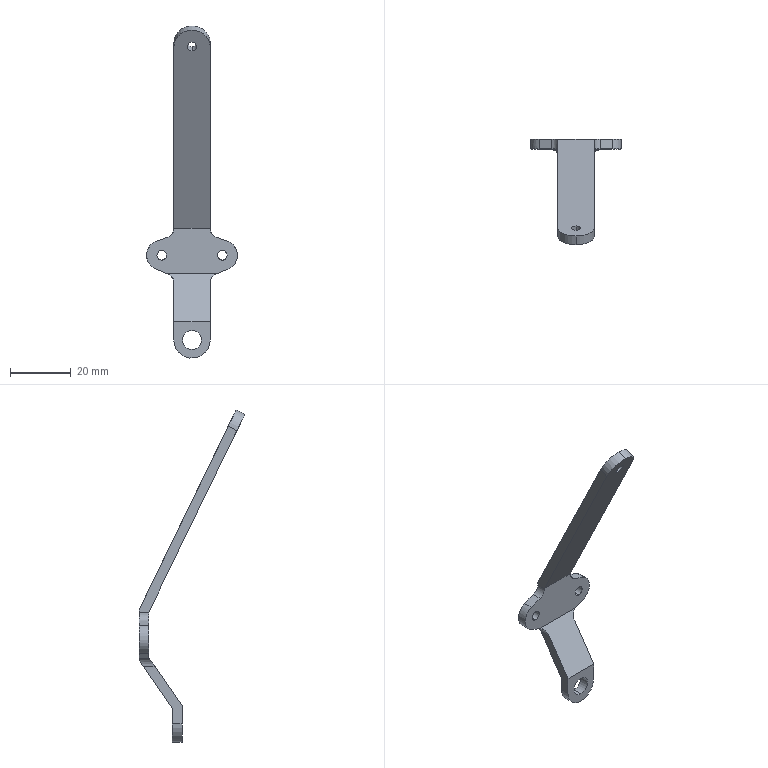Part | SolidWorks | features BaseBody 1 | 1 solid | 33 faces | box 30 x 34.955 x 109.796 mm | volume 4900 mm3 | cylinder 17 | plane 16 | commonest cylinder face diameters 3.2 x6 6 x4 12 x3 6.261 x2 10 x2
STEP:
#1=CARTESIAN_POINT('',(0.,-11.,-24.87));
#2=VERTEX_POINT('',#1);
#3=CARTESIAN_POINT('',(0.,-11.,-31.13));
#4=VERTEX_POINT('',#3);
#5=CARTESIAN_POINT('',(0.,-11.,-28.));
#6=DIRECTION('',(0.,-1.,0.));
#7=DIRECTION('',(0.,0.,1.));
#8=AXIS2_PLACEMENT_3D('',#5,#6,#7);
#9=CIRCLE('',#8,3.13);
#10=EDGE_CURVE('',#2,#4,#9,.T.);
#11=ORIENTED_EDGE('',*,*,#10,.T.);
#12=CARTESIAN_POINT('',(0.,-7.8,-31.13));
#13=VERTEX_POINT('',#12);
#14=CARTESIAN_POINT('',(0.,-11.,-31.13));
#15=DIRECTION('',(0.,1.,0.));
#16=VECTOR('',#15,1000.);
#17=LINE('',#14,#16);
#18=EDGE_CURVE('',#4,#13,#17,.T.);
#19=ORIENTED_EDGE('',*,*,#18,.T.);
#20=CARTESIAN_POINT('',(0.,-7.8,-24.87));
#21=VERTEX_POINT('',#20);
#22=CARTESIAN_POINT('',(0.,-7.8,-28.));
#23=DIRECTION('',(0.,1.,0.));
#24=DIRECTION('',(0.,0.,1.));
#25=AXIS2_PLACEMENT_3D('',#22,#23,#24);
#26=CIRCLE('',#25,3.13);
#27=EDGE_CURVE('',#13,#21,#26,.T.);
#28=ORIENTED_EDGE('',*,*,#27,.T.);
#29=CARTESIAN_POINT('',(0.,-11.,-24.87));
#30=DIRECTION('',(0.,1.,0.));
#31=VECTOR('',#30,1000.);
#32=LINE('',#29,#31);
#33=EDGE_CURVE('',#2,#21,#32,.T.);
#34=ORIENTED_EDGE('',*,*,#33,.F.);
#35=EDGE_LOOP('',(#11,#19,#28,#34));
#36=FACE_OUTER_BOUND('',#35,.T.);
#37=CARTESIAN_POINT('',(0.,-11.,-28.));
#38=DIRECTION('',(0.,1.,0.));
#39=DIRECTION('',(0.,0.,1.));
#40=AXIS2_PLACEMENT_3D('',#37,#38,#39);
#41=CYLINDRICAL_SURFACE('',#40,3.13);
#42=ADVANCED_FACE('',(#36),#41,.F.);
#43=CARTESIAN_POINT('',(-10.,0.,1.6));
#44=VERTEX_POINT('',#43);
#45=CARTESIAN_POINT('',(-10.,0.,-1.6));
#46=VERTEX_POINT('',#45);
#47=CARTESIAN_POINT('',(-10.,0.,1.6));
#48=CARTESIAN_POINT('',(-13.2,0.,1.6));
#49=CARTESIAN_POINT('',(-13.2,0.,-1.6));
#50=CARTESIAN_POINT('',(-10.,0.,-1.6));
#51=(BOUNDED_CURVE()B_SPLINE_CURVE(3,(#47,#48,#49,#50),.UNSPECIFIED.,.F.,.F.)B_SPLINE_CURVE_WITH_KNOTS((4,4),(0.,3.142),.UNSPECIFIED.)CURVE()GEOMETRIC_REPRESENTATION_ITEM()RATIONAL_B_SPLINE_CURVE((1.,0.3333,0.3333,1.))REPRESENTATION_ITEM(''));
#52=EDGE_CURVE('',#44,#46,#51,.T.);
#53=ORIENTED_EDGE('',*,*,#52,.T.);
#54=CARTESIAN_POINT('',(-10.,3.193,-1.596));
#55=VERTEX_POINT('',#54);
#56=CARTESIAN_POINT('',(-10.,-0.01916,-1.6));
#57=DIRECTION('',(0.,1.,0.001373));
#58=VECTOR('',#57,1000.);
#59=LINE('',#56,#58);
#60=EDGE_CURVE('',#46,#55,#59,.T.);
#61=ORIENTED_EDGE('',*,*,#60,.T.);
#62=CARTESIAN_POINT('',(-10.,3.188,1.604));
#63=VERTEX_POINT('',#62);
#64=CARTESIAN_POINT('',(-10.,3.19,0.004381));
#65=DIRECTION('',(0.,1.,0.001373));
#66=DIRECTION('',(0.,-0.001373,1.));
#67=AXIS2_PLACEMENT_3D('',#64,#65,#66);
#68=CIRCLE('',#67,1.6);
#69=EDGE_CURVE('',#55,#63,#68,.T.);
#70=ORIENTED_EDGE('',*,*,#69,.T.);
#71=CARTESIAN_POINT('',(-10.,-0.02355,1.6));
#72=DIRECTION('',(0.,1.,0.001373));
#73=VECTOR('',#72,1000.);
#74=LINE('',#71,#73);
#75=EDGE_CURVE('',#44,#63,#74,.T.);
#76=ORIENTED_EDGE('',*,*,#75,.F.);
#77=EDGE_LOOP('',(#53,#61,#70,#76));
#78=FACE_OUTER_BOUND('',#77,.T.);
#79=CARTESIAN_POINT('',(-10.,-0.02135,-0.00002932));
#80=DIRECTION('',(0.,1.,0.001373));
#81=DIRECTION('',(0.,-0.001373,1.));
#82=AXIS2_PLACEMENT_3D('',#79,#80,#81);
#83=CYLINDRICAL_SURFACE('',#82,1.6);
#84=ADVANCED_FACE('',(#78),#83,.F.);
#85=CARTESIAN_POINT('',(10.,0.,1.6));
#86=VERTEX_POINT('',#85);
#87=CARTESIAN_POINT('',(10.,0.,-1.6));
#88=VERTEX_POINT('',#87);
#89=CARTESIAN_POINT('',(10.,0.,1.6));
#90=CARTESIAN_POINT('',(6.8,0.,1.6));
#91=CARTESIAN_POINT('',(6.8,0.,-1.6));
#92=CARTESIAN_POINT('',(10.,0.,-1.6));
#93=(BOUNDED_CURVE()B_SPLINE_CURVE(3,(#89,#90,#91,#92),.UNSPECIFIED.,.F.,.F.)B_SPLINE_CURVE_WITH_KNOTS((4,4),(0.,3.142),.UNSPECIFIED.)CURVE()GEOMETRIC_REPRESENTATION_ITEM()RATIONAL_B_SPLINE_CURVE((1.,0.3333,0.3333,1.))REPRESENTATION_ITEM(''));
#94=EDGE_CURVE('',#86,#88,#93,.T.);
#95=ORIENTED_EDGE('',*,*,#94,.T.);
#96=CARTESIAN_POINT('',(10.,3.193,-1.596));
#97=VERTEX_POINT('',#96);
#98=CARTESIAN_POINT('',(10.,-0.01916,-1.6));
#99=DIRECTION('',(0.,1.,0.001373));
#100=VECTOR('',#99,1000.);
#101=LINE('',#98,#100);
#102=EDGE_CURVE('',#88,#97,#101,.T.);
#103=ORIENTED_EDGE('',*,*,#102,.T.);
#104=CARTESIAN_POINT('',(10.,3.188,1.604));
#105=VERTEX_POINT('',#104);
#106=CARTESIAN_POINT('',(10.,3.19,0.004381));
#107=DIRECTION('',(0.,1.,0.001373));
#108=DIRECTION('',(0.,-0.001373,1.));
#109=AXIS2_PLACEMENT_3D('',#106,#107,#108);
#110=CIRCLE('',#109,1.6);
#111=EDGE_CURVE('',#97,#105,#110,.T.);
#112=ORIENTED_EDGE('',*,*,#111,.T.);
#113=CARTESIAN_POINT('',(10.,-0.02355,1.6));
#114=DIRECTION('',(0.,1.,0.001373));
#115=VECTOR('',#114,1000.);
#116=LINE('',#113,#115);
#117=EDGE_CURVE('',#86,#105,#116,.T.);
#118=ORIENTED_EDGE('',*,*,#117,.F.);
#119=EDGE_LOOP('',(#95,#103,#112,#118));
#120=FACE_OUTER_BOUND('',#119,.T.);
#121=CARTESIAN_POINT('',(10.,-0.02135,-0.00002932));
#122=DIRECTION('',(0.,1.,0.001373));
#123=DIRECTION('',(0.,-0.001373,1.));
#124=AXIS2_PLACEMENT_3D('',#121,#122,#123);
#125=CYLINDRICAL_SURFACE('',#124,1.6);
#126=ADVANCED_FACE('',(#120),#125,.F.);
#127=CARTESIAN_POINT('',(0.,-29.834,70.44));
#128=VERTEX_POINT('',#127);
#129=CARTESIAN_POINT('',(0.,-28.436,67.561));
#130=VERTEX_POINT('',#129);
#131=CARTESIAN_POINT('',(0.,-29.135,69.001));
#132=DIRECTION('',(0.,-0.8996,-0.4368));
#133=DIRECTION('',(0.,-0.4368,0.8996));
#134=AXIS2_PLACEMENT_3D('',#131,#132,#133);
#135=CIRCLE('',#134,1.6);
#136=EDGE_CURVE('',#128,#130,#135,.T.);
#137=ORIENTED_EDGE('',*,*,#136,.T.);
#138=CARTESIAN_POINT('',(0.,-25.557,68.959));
#139=VERTEX_POINT('',#138);
#140=CARTESIAN_POINT('',(0.,-28.436,67.561));
#141=DIRECTION('',(0.,0.8996,0.4368));
#142=VECTOR('',#141,1000.);
#143=LINE('',#140,#142);
#144=EDGE_CURVE('',#130,#139,#143,.T.);
#145=ORIENTED_EDGE('',*,*,#144,.T.);
#146=CARTESIAN_POINT('',(0.,-26.955,71.838));
#147=VERTEX_POINT('',#146);
#148=CARTESIAN_POINT('',(0.,-26.256,70.398));
#149=DIRECTION('',(0.,0.8996,0.4368));
#150=DIRECTION('',(0.,-0.4368,0.8996));
#151=AXIS2_PLACEMENT_3D('',#148,#149,#150);
#152=CIRCLE('',#151,1.6);
#153=EDGE_CURVE('',#139,#147,#152,.T.);
#154=ORIENTED_EDGE('',*,*,#153,.T.);
#155=CARTESIAN_POINT('',(0.,-29.834,70.44));
#156=DIRECTION('',(0.,0.8996,0.4368));
#157=VECTOR('',#156,1000.);
#158=LINE('',#155,#157);
#159=EDGE_CURVE('',#128,#147,#158,.T.);
#160=ORIENTED_EDGE('',*,*,#159,.F.);
#161=EDGE_LOOP('',(#137,#145,#154,#160));
#162=FACE_OUTER_BOUND('',#161,.T.);
#163=CARTESIAN_POINT('',(0.,-29.135,69.001));
#164=DIRECTION('',(0.,0.8996,0.4368));
#165=DIRECTION('',(0.,-0.4368,0.8996));
#166=AXIS2_PLACEMENT_3D('',#163,#164,#165);
#167=CYLINDRICAL_SURFACE('',#166,1.6);
#168=ADVANCED_FACE('',(#162),#167,.F.);
#169=CARTESIAN_POINT('',(-6.,-29.135,69.001));
#170=VERTEX_POINT('',#169);
#171=CARTESIAN_POINT('',(0.,-31.755,74.398));
#172=VERTEX_POINT('',#171);
#173=CARTESIAN_POINT('',(0.,-29.135,69.001));
#174=DIRECTION('',(0.,0.8996,0.4368));
#175=DIRECTION('',(0.,-0.4368,0.8996));
#176=AXIS2_PLACEMENT_3D('',#173,#174,#175);
#177=CIRCLE('',#176,6.);
#178=EDGE_CURVE('',#170,#172,#177,.T.);
#179=ORIENTED_EDGE('',*,*,#178,.T.);
#180=CARTESIAN_POINT('',(0.,-28.877,75.796));
#181=VERTEX_POINT('',#180);
#182=CARTESIAN_POINT('',(0.,-31.755,74.398));
#183=DIRECTION('',(0.,0.8996,0.4368));
#184=VECTOR('',#183,1000.);
#185=LINE('',#182,#184);
#186=EDGE_CURVE('',#172,#181,#185,.T.);
#187=ORIENTED_EDGE('',*,*,#186,.T.);
#188=CARTESIAN_POINT('',(-6.,-26.256,70.398));
#189=VERTEX_POINT('',#188);
#190=CARTESIAN_POINT('',(0.,-26.256,70.398));
#191=DIRECTION('',(0.,-0.8996,-0.4368));
#192=DIRECTION('',(0.,-0.4368,0.8996));
#193=AXIS2_PLACEMENT_3D('',#190,#191,#192);
#194=CIRCLE('',#193,6.);
#195=EDGE_CURVE('',#181,#189,#194,.T.);
#196=ORIENTED_EDGE('',*,*,#195,.T.);
#197=CARTESIAN_POINT('',(-6.,-29.135,69.001));
#198=DIRECTION('',(0.,0.8996,0.4368));
#199=VECTOR('',#198,1000.);
#200=LINE('',#197,#199);
#201=EDGE_CURVE('',#170,#189,#200,.T.);
#202=ORIENTED_EDGE('',*,*,#201,.F.);
#203=EDGE_LOOP('',(#179,#187,#196,#202));
#204=FACE_OUTER_BOUND('',#203,.T.);
#205=CARTESIAN_POINT('',(0.,-29.135,69.001));
#206=DIRECTION('',(0.,0.8996,0.4368));
#207=DIRECTION('',(0.,-0.4368,0.8996));
#208=AXIS2_PLACEMENT_3D('',#205,#206,#207);
#209=CYLINDRICAL_SURFACE('',#208,6.);
#210=ADVANCED_FACE('',(#204),#209,.T.);
#211=ORIENTED_EDGE('',*,*,#18,.F.);
#212=CARTESIAN_POINT('',(0.,-11.,-28.));
#213=DIRECTION('',(0.,-1.,0.));
#214=DIRECTION('',(0.,0.,1.));
#215=AXIS2_PLACEMENT_3D('',#212,#213,#214);
#216=CIRCLE('',#215,3.13);
#217=EDGE_CURVE('',#4,#2,#216,.T.);
#218=ORIENTED_EDGE('',*,*,#217,.T.);
#219=ORIENTED_EDGE('',*,*,#33,.T.);
#220=CARTESIAN_POINT('',(0.,-7.8,-28.));
#221=DIRECTION('',(0.,1.,0.));
#222=DIRECTION('',(0.,0.,1.));
#223=AXIS2_PLACEMENT_3D('',#220,#221,#222);
#224=CIRCLE('',#223,3.13);
#225=EDGE_CURVE('',#21,#13,#224,.T.);
#226=ORIENTED_EDGE('',*,*,#225,.T.);
#227=EDGE_LOOP('',(#211,#218,#219,#226));
#228=FACE_OUTER_BOUND('',#227,.T.);
#229=CARTESIAN_POINT('',(0.,-11.,-28.));
#230=DIRECTION('',(0.,1.,0.));
#231=DIRECTION('',(0.,0.,1.));
#232=AXIS2_PLACEMENT_3D('',#229,#230,#231);
#233=CYLINDRICAL_SURFACE('',#232,3.13);
#234=ADVANCED_FACE('',(#228),#233,.F.);
#235=ORIENTED_EDGE('',*,*,#225,.F.);
#236=ORIENTED_EDGE('',*,*,#27,.F.);
#237=EDGE_LOOP('',(#235,#236));
#238=FACE_BOUND('',#237,.T.);
#239=CARTESIAN_POINT('',(-6.,-7.8,-22.994));
#240=VERTEX_POINT('',#239);
#241=CARTESIAN_POINT('',(-6.,-7.8,-28.));
#242=VERTEX_POINT('',#241);
#243=CARTESIAN_POINT('',(-6.,-7.8,-28.53));
#244=DIRECTION('',(0.,0.,-1.));
#245=VECTOR('',#244,1000.);
#246=LINE('',#243,#245);
#247=EDGE_CURVE('',#240,#242,#246,.T.);
#248=ORIENTED_EDGE('',*,*,#247,.F.);
#249=CARTESIAN_POINT('',(6.,-7.8,-22.994));
#250=VERTEX_POINT('',#249);
#251=CARTESIAN_POINT('',(0.,-7.8,-22.994));
#252=DIRECTION('',(-1.,0.,0.));
#253=VECTOR('',#252,1000.);
#254=LINE('',#251,#253);
#255=EDGE_CURVE('',#250,#240,#254,.T.);
#256=ORIENTED_EDGE('',*,*,#255,.F.);
#257=CARTESIAN_POINT('',(6.,-7.8,-28.));
#258=VERTEX_POINT('',#257);
#259=CARTESIAN_POINT('',(6.,-7.8,-28.53));
#260=DIRECTION('',(0.,0.,1.));
#261=VECTOR('',#260,1000.);
#262=LINE('',#259,#261);
#263=EDGE_CURVE('',#258,#250,#262,.T.);
#264=ORIENTED_EDGE('',*,*,#263,.F.);
#265=CARTESIAN_POINT('',(0.,-7.8,-28.));
#266=DIRECTION('',(0.,-1.,0.));
#267=DIRECTION('',(0.,0.,1.));
#268=AXIS2_PLACEMENT_3D('',#265,#266,#267);
#269=CIRCLE('',#268,6.);
#270=EDGE_CURVE('',#242,#258,#269,.T.);
#271=ORIENTED_EDGE('',*,*,#270,.F.);
#272=EDGE_LOOP('',(#248,#256,#264,#271));
#273=FACE_OUTER_BOUND('',#272,.T.);
#274=CARTESIAN_POINT('',(-6.,-7.8,-22.994));
#275=DIRECTION('',(0.,-1.,0.));
#276=DIRECTION('',(0.,0.,-1.));
#277=AXIS2_PLACEMENT_3D('',#274,#275,#276);
#278=PLANE('',#277);
#279=ADVANCED_FACE('',(#238,#273),#278,.F.);
#280=ORIENTED_EDGE('',*,*,#10,.F.);
#281=ORIENTED_EDGE('',*,*,#217,.F.);
#282=EDGE_LOOP('',(#280,#281));
#283=FACE_BOUND('',#282,.T.);
#284=CARTESIAN_POINT('',(6.,-11.,-28.));
#285=VERTEX_POINT('',#284);
#286=CARTESIAN_POINT('',(-6.,-11.,-28.));
#287=VERTEX_POINT('',#286);
#288=CARTESIAN_POINT('',(0.,-11.,-28.));
#289=DIRECTION('',(0.,1.,0.));
#290=DIRECTION('',(0.,0.,1.));
#291=AXIS2_PLACEMENT_3D('',#288,#289,#290);
#292=CIRCLE('',#291,6.);
#293=EDGE_CURVE('',#285,#287,#292,.T.);
#294=ORIENTED_EDGE('',*,*,#293,.F.);
#295=CARTESIAN_POINT('',(6.,-11.,-22.));
#296=VERTEX_POINT('',#295);
#297=CARTESIAN_POINT('',(6.,-11.,-28.036));
#298=DIRECTION('',(0.,0.,-1.));
#299=VECTOR('',#298,1000.);
#300=LINE('',#297,#299);
#301=EDGE_CURVE('',#296,#285,#300,.T.);
#302=ORIENTED_EDGE('',*,*,#301,.F.);
#303=CARTESIAN_POINT('',(-6.,-11.,-22.));
#304=VERTEX_POINT('',#303);
#305=CARTESIAN_POINT('',(0.,-11.,-22.));
#306=DIRECTION('',(1.,0.,0.));
#307=VECTOR('',#306,1000.);
#308=LINE('',#305,#307);
#309=EDGE_CURVE('',#304,#296,#308,.T.);
#310=ORIENTED_EDGE('',*,*,#309,.F.);
#311=CARTESIAN_POINT('',(-6.,-11.,-28.036));
#312=DIRECTION('',(0.,0.,1.));
#313=VECTOR('',#312,1000.);
#314=LINE('',#311,#313);
#315=EDGE_CURVE('',#287,#304,#314,.T.);
#316=ORIENTED_EDGE('',*,*,#315,.F.);
#317=EDGE_LOOP('',(#294,#302,#310,#316));
#318=FACE_OUTER_BOUND('',#317,.T.);
#319=CARTESIAN_POINT('',(-6.,-11.,-34.072));
#320=DIRECTION('',(0.,1.,0.));
#321=DIRECTION('',(0.,0.,1.));
#322=AXIS2_PLACEMENT_3D('',#319,#320,#321);
#323=PLANE('',#322);
#324=ADVANCED_FACE('',(#283,#318),#323,.F.);
#325=ORIENTED_EDGE('',*,*,#270,.T.);
#326=CARTESIAN_POINT('',(6.,-9.4,-28.));
#327=DIRECTION('',(0.,1.,0.));
#328=VECTOR('',#327,1000.);
#329=LINE('',#326,#328);
#330=EDGE_CURVE('',#285,#258,#329,.T.);
#331=ORIENTED_EDGE('',*,*,#330,.F.);
#332=ORIENTED_EDGE('',*,*,#293,.T.);
#333=CARTESIAN_POINT('',(-6.,-9.4,-28.));
#334=DIRECTION('',(0.,-1.,0.));
#335=VECTOR('',#334,1000.);
#336=LINE('',#333,#335);
#337=EDGE_CURVE('',#242,#287,#336,.T.);
#338=ORIENTED_EDGE('',*,*,#337,.F.);
#339=EDGE_LOOP('',(#325,#331,#332,#338));
#340=FACE_OUTER_BOUND('',#339,.T.);
#341=CARTESIAN_POINT('',(0.,-11.,-28.));
#342=DIRECTION('',(0.,1.,0.));
#343=DIRECTION('',(0.,0.,1.));
#344=AXIS2_PLACEMENT_3D('',#341,#342,#343);
#345=CYLINDRICAL_SURFACE('',#344,6.);
#346=ADVANCED_FACE('',(#340),#345,.T.);
#347=CARTESIAN_POINT('',(-6.,1.807,-9.02));
#348=VERTEX_POINT('',#347);
#349=CARTESIAN_POINT('',(-6.,1.807,-9.02));
#350=DIRECTION('',(0.,-0.5665,-0.824));
#351=VECTOR('',#350,1000.);
#352=LINE('',#349,#351);
#353=EDGE_CURVE('',#348,#240,#352,.T.);
#354=ORIENTED_EDGE('',*,*,#353,.T.);
#355=ORIENTED_EDGE('',*,*,#247,.T.);
#356=ORIENTED_EDGE('',*,*,#337,.T.);
#357=ORIENTED_EDGE('',*,*,#315,.T.);
#358=CARTESIAN_POINT('',(-6.,-2.08,-9.025));
#359=VERTEX_POINT('',#358);
#360=CARTESIAN_POINT('',(-6.,-11.,-22.));
#361=DIRECTION('',(0.,0.5665,0.824));
#362=VECTOR('',#361,1000.);
#363=LINE('',#360,#362);
#364=EDGE_CURVE('',#304,#359,#363,.T.);
#365=ORIENTED_EDGE('',*,*,#364,.T.);
#366=CARTESIAN_POINT('',(-6.,-2.08,-9.025));
#367=DIRECTION('',(0.,1.,0.001373));
#368=VECTOR('',#367,1000.);
#369=LINE('',#366,#368);
#370=EDGE_CURVE('',#359,#348,#369,.T.);
#371=ORIENTED_EDGE('',*,*,#370,.T.);
#372=EDGE_LOOP('',(#354,#355,#356,#357,#365,#371));
#373=FACE_OUTER_BOUND('',#372,.T.);
#374=CARTESIAN_POINT('',(-6.,-11.,-28.));
#375=DIRECTION('',(-1.,0.,0.));
#376=DIRECTION('',(0.,0.,1.));
#377=AXIS2_PLACEMENT_3D('',#374,#375,#376);
#378=PLANE('',#377);
#379=ADVANCED_FACE('',(#373),#378,.T.);
#380=CARTESIAN_POINT('',(-6.786,3.2,-6.994));
#381=VERTEX_POINT('',#380);
#382=CARTESIAN_POINT('',(-6.786,3.2,-6.994));
#383=CARTESIAN_POINT('',(-6.274,2.815,-7.554));
#384=CARTESIAN_POINT('',(-6.,2.329,-8.261));
#385=CARTESIAN_POINT('',(-6.,1.807,-9.02));
#386=(BOUNDED_CURVE()B_SPLINE_CURVE(3,(#382,#383,#384,#385),.UNSPECIFIED.,.F.,.F.)B_SPLINE_CURVE_WITH_KNOTS((4,4),(0.8303,1.571),.UNSPECIFIED.)CURVE()GEOMETRIC_REPRESENTATION_ITEM()RATIONAL_B_SPLINE_CURVE((1.,0.9548,0.9548,1.))REPRESENTATION_ITEM(''));
#387=EDGE_CURVE('',#381,#348,#386,.T.);
#388=ORIENTED_EDGE('',*,*,#387,.F.);
#389=CARTESIAN_POINT('',(6.786,3.2,-6.994));
#390=VERTEX_POINT('',#389);
#391=CARTESIAN_POINT('',(0.,3.2,-6.994));
#392=DIRECTION('',(-1.,0.,0.));
#393=VECTOR('',#392,1000.);
#394=LINE('',#391,#393);
#395=EDGE_CURVE('',#390,#381,#394,.T.);
#396=ORIENTED_EDGE('',*,*,#395,.F.);
#397=CARTESIAN_POINT('',(6.,1.807,-9.02));
#398=VERTEX_POINT('',#397);
#399=CARTESIAN_POINT('',(6.,1.807,-9.02));
#400=CARTESIAN_POINT('',(6.,2.329,-8.261));
#401=CARTESIAN_POINT('',(6.274,2.815,-7.554));
#402=CARTESIAN_POINT('',(6.786,3.2,-6.994));
#403=(BOUNDED_CURVE()B_SPLINE_CURVE(3,(#399,#400,#401,#402),.UNSPECIFIED.,.F.,.F.)B_SPLINE_CURVE_WITH_KNOTS((4,4),(4.712,5.453),.UNSPECIFIED.)CURVE()GEOMETRIC_REPRESENTATION_ITEM()RATIONAL_B_SPLINE_CURVE((1.,0.9548,0.9548,1.))REPRESENTATION_ITEM(''));
#404=EDGE_CURVE('',#398,#390,#403,.T.);
#405=ORIENTED_EDGE('',*,*,#404,.F.);
#406=CARTESIAN_POINT('',(6.,-2.3,-14.994));
#407=DIRECTION('',(0.,0.5665,0.824));
#408=VECTOR('',#407,1000.);
#409=LINE('',#406,#408);
#410=EDGE_CURVE('',#250,#398,#409,.T.);
#411=ORIENTED_EDGE('',*,*,#410,.F.);
#412=ORIENTED_EDGE('',*,*,#255,.T.);
#413=ORIENTED_EDGE('',*,*,#353,.F.);
#414=EDGE_LOOP('',(#388,#396,#405,#411,#412,#413));
#415=FACE_OUTER_BOUND('',#414,.T.);
#416=CARTESIAN_POINT('',(-6.867,3.2,-6.994));
#417=DIRECTION('',(0.,-0.824,0.5665));
#418=DIRECTION('',(0.,-0.5665,-0.824));
#419=AXIS2_PLACEMENT_3D('',#416,#417,#418);
#420=PLANE('',#419);
#421=ADVANCED_FACE('',(#415),#420,.F.);
#422=ORIENTED_EDGE('',*,*,#330,.T.);
#423=ORIENTED_EDGE('',*,*,#263,.T.);
#424=ORIENTED_EDGE('',*,*,#410,.T.);
#425=CARTESIAN_POINT('',(6.,-2.08,-9.025));
#426=VERTEX_POINT('',#425);
#427=CARTESIAN_POINT('',(6.,-2.111,-9.025));
#428=DIRECTION('',(0.,1.,0.001373));
#429=VECTOR('',#428,1000.);
#430=LINE('',#427,#429);
#431=EDGE_CURVE('',#426,#398,#430,.T.);
#432=ORIENTED_EDGE('',*,*,#431,.F.);
#433=CARTESIAN_POINT('',(6.,-11.,-22.));
#434=DIRECTION('',(0.,0.5665,0.824));
#435=VECTOR('',#434,1000.);
#436=LINE('',#433,#435);
#437=EDGE_CURVE('',#296,#426,#436,.T.);
#438=ORIENTED_EDGE('',*,*,#437,.F.);
#439=ORIENTED_EDGE('',*,*,#301,.T.);
#440=EDGE_LOOP('',(#422,#423,#424,#432,#438,#439));
#441=FACE_OUTER_BOUND('',#440,.T.);
#442=CARTESIAN_POINT('',(6.,-11.,-28.));
#443=DIRECTION('',(-1.,0.,0.));
#444=DIRECTION('',(0.,0.,1.));
#445=AXIS2_PLACEMENT_3D('',#442,#443,#444);
#446=PLANE('',#445);
#447=ADVANCED_FACE('',(#441),#446,.F.);
#448=ORIENTED_EDGE('',*,*,#309,.T.);
#449=ORIENTED_EDGE('',*,*,#437,.T.);
#450=CARTESIAN_POINT('',(7.882,-0.1639,-6.238));
#451=VERTEX_POINT('',#450);
#452=CARTESIAN_POINT('',(7.882,-0.1639,-6.238));
#453=CARTESIAN_POINT('',(6.708,-0.4882,-6.71));
#454=CARTESIAN_POINT('',(6.,-1.209,-7.759));
#455=CARTESIAN_POINT('',(6.,-2.08,-9.025));
#456=(BOUNDED_CURVE()B_SPLINE_CURVE(3,(#452,#453,#454,#455),.UNSPECIFIED.,.F.,.F.)B_SPLINE_CURVE_WITH_KNOTS((4,4),(0.3818,1.571),.UNSPECIFIED.)CURVE()GEOMETRIC_REPRESENTATION_ITEM()RATIONAL_B_SPLINE_CURVE((1.,0.8856,0.8856,1.))REPRESENTATION_ITEM(''));
#457=EDGE_CURVE('',#451,#426,#456,.T.);
#458=ORIENTED_EDGE('',*,*,#457,.F.);
#459=CARTESIAN_POINT('',(8.476,0.,-6.));
#460=VERTEX_POINT('',#459);
#461=CARTESIAN_POINT('',(7.882,-0.1639,-6.238));
#462=DIRECTION('',(0.8988,0.2483,0.3612));
#463=VECTOR('',#462,1000.);
#464=LINE('',#461,#463);
#465=EDGE_CURVE('',#451,#460,#464,.T.);
#466=ORIENTED_EDGE('',*,*,#465,.T.);
#467=CARTESIAN_POINT('',(-8.476,0.,-6.));
#468=VERTEX_POINT('',#467);
#469=CARTESIAN_POINT('',(0.,0.,-6.));
#470=DIRECTION('',(1.,0.,0.));
#471=VECTOR('',#470,1000.);
#472=LINE('',#469,#471);
#473=EDGE_CURVE('',#468,#460,#472,.T.);
#474=ORIENTED_EDGE('',*,*,#473,.F.);
#475=CARTESIAN_POINT('',(-7.882,-0.1639,-6.238));
#476=VERTEX_POINT('',#475);
#477=CARTESIAN_POINT('',(-7.882,-0.1639,-6.238));
#478=DIRECTION('',(-0.8988,0.2483,0.3612));
#479=VECTOR('',#478,1000.);
#480=LINE('',#477,#479);
#481=EDGE_CURVE('',#476,#468,#480,.T.);
#482=ORIENTED_EDGE('',*,*,#481,.F.);
#483=CARTESIAN_POINT('',(-6.,-2.08,-9.025));
#484=CARTESIAN_POINT('',(-6.,-1.209,-7.759));
#485=CARTESIAN_POINT('',(-6.708,-0.4882,-6.71));
#486=CARTESIAN_POINT('',(-7.882,-0.1639,-6.238));
#487=(BOUNDED_CURVE()B_SPLINE_CURVE(3,(#483,#484,#485,#486),.UNSPECIFIED.,.F.,.F.)B_SPLINE_CURVE_WITH_KNOTS((4,4),(4.712,5.901),.UNSPECIFIED.)CURVE()GEOMETRIC_REPRESENTATION_ITEM()RATIONAL_B_SPLINE_CURVE((1.,0.8856,0.8856,1.))REPRESENTATION_ITEM(''));
#488=EDGE_CURVE('',#359,#476,#487,.T.);
#489=ORIENTED_EDGE('',*,*,#488,.F.);
#490=ORIENTED_EDGE('',*,*,#364,.F.);
#491=EDGE_LOOP('',(#448,#449,#458,#466,#474,#482,#489,#490));
#492=FACE_OUTER_BOUND('',#491,.T.);
#493=CARTESIAN_POINT('',(-8.577,-11.,-22.));
#494=DIRECTION('',(0.,0.824,-0.5665));
#495=DIRECTION('',(0.,0.5665,0.824));
#496=AXIS2_PLACEMENT_3D('',#493,#494,#495);
#497=PLANE('',#496);
#498=ADVANCED_FACE('',(#492),#497,.F.);
#499=CARTESIAN_POINT('',(-7.882,3.199,-6.234));
#500=VERTEX_POINT('',#499);
#501=CARTESIAN_POINT('',(-9.,3.203,-9.018));
#502=DIRECTION('',(0.,1.,0.001373));
#503=DIRECTION('',(0.,-0.001373,1.));
#504=AXIS2_PLACEMENT_3D('',#501,#502,#503);
#505=CIRCLE('',#504,3.);
#506=EDGE_CURVE('',#500,#381,#505,.T.);
#507=ORIENTED_EDGE('',*,*,#506,.T.);
#508=ORIENTED_EDGE('',*,*,#387,.T.);
#509=ORIENTED_EDGE('',*,*,#370,.F.);
#510=ORIENTED_EDGE('',*,*,#488,.T.);
#511=CARTESIAN_POINT('',(-7.882,0.5419,-6.237));
#512=DIRECTION('',(0.,1.,0.001373));
#513=VECTOR('',#512,1000.);
#514=LINE('',#511,#513);
#515=EDGE_CURVE('',#476,#500,#514,.T.);
#516=ORIENTED_EDGE('',*,*,#515,.T.);
#517=EDGE_LOOP('',(#507,#508,#509,#510,#516));
#518=FACE_OUTER_BOUND('',#517,.T.);
#519=CARTESIAN_POINT('',(-9.,-2.111,-9.025));
#520=DIRECTION('',(0.,1.,0.001373));
#521=DIRECTION('',(0.,-0.001373,1.));
#522=AXIS2_PLACEMENT_3D('',#519,#520,#521);
#523=CYLINDRICAL_SURFACE('',#522,3.);
#524=ADVANCED_FACE('',(#518),#523,.F.);
#525=CARTESIAN_POINT('',(-10.,3.19,0.004381));
#526=DIRECTION('',(0.,1.,0.001373));
#527=DIRECTION('',(0.,-0.001373,1.));
#528=AXIS2_PLACEMENT_3D('',#525,#526,#527);
#529=CIRCLE('',#528,1.6);
#530=EDGE_CURVE('',#63,#55,#529,.T.);
#531=ORIENTED_EDGE('',*,*,#530,.F.);
#532=ORIENTED_EDGE('',*,*,#69,.F.);
#533=EDGE_LOOP('',(#531,#532));
#534=FACE_BOUND('',#533,.T.);
#535=CARTESIAN_POINT('',(10.,3.19,0.004381));
#536=DIRECTION('',(0.,1.,0.001373));
#537=DIRECTION('',(0.,-0.001373,1.));
#538=AXIS2_PLACEMENT_3D('',#535,#536,#537);
#539=CIRCLE('',#538,1.6);
#540=EDGE_CURVE('',#105,#97,#539,.T.);
#541=ORIENTED_EDGE('',*,*,#540,.F.);
#542=ORIENTED_EDGE('',*,*,#111,.F.);
#543=EDGE_LOOP('',(#541,#542));
#544=FACE_BOUND('',#543,.T.);
#545=ORIENTED_EDGE('',*,*,#506,.F.);
#546=CARTESIAN_POINT('',(-11.863,3.197,-4.636));
#547=VERTEX_POINT('',#546);
#548=CARTESIAN_POINT('',(-11.863,3.197,-4.636));
#549=DIRECTION('',(0.928,0.0005116,-0.3726));
#550=VECTOR('',#549,1000.);
#551=LINE('',#548,#550);
#552=EDGE_CURVE('',#547,#500,#551,.T.);
#553=ORIENTED_EDGE('',*,*,#552,.F.);
#554=CARTESIAN_POINT('',(-12.184,3.184,4.502));
#555=VERTEX_POINT('',#554);
#556=CARTESIAN_POINT('',(-10.,3.19,0.004381));
#557=DIRECTION('',(0.,-1.,-0.001373));
#558=DIRECTION('',(0.,-0.001373,1.));
#559=AXIS2_PLACEMENT_3D('',#556,#557,#558);
#560=CIRCLE('',#559,5.);
#561=EDGE_CURVE('',#555,#547,#560,.T.);
#562=ORIENTED_EDGE('',*,*,#561,.F.);
#563=CARTESIAN_POINT('',(-8.,3.182,5.981));
#564=VERTEX_POINT('',#563);
#565=CARTESIAN_POINT('',(-8.,3.182,5.981));
#566=DIRECTION('',(-0.9429,0.0004575,-0.3332));
#567=VECTOR('',#566,1000.);
#568=LINE('',#565,#567);
#569=EDGE_CURVE('',#564,#555,#568,.T.);
#570=ORIENTED_EDGE('',*,*,#569,.F.);
#571=CARTESIAN_POINT('',(-6.,3.178,8.809));
#572=VERTEX_POINT('',#571);
#573=CARTESIAN_POINT('',(-9.,3.178,8.809));
#574=DIRECTION('',(0.,1.,0.001373));
#575=DIRECTION('',(0.,-0.001373,1.));
#576=AXIS2_PLACEMENT_3D('',#573,#574,#575);
#577=CIRCLE('',#576,3.);
#578=EDGE_CURVE('',#572,#564,#577,.T.);
#579=ORIENTED_EDGE('',*,*,#578,.F.);
#580=CARTESIAN_POINT('',(-6.,3.177,9.783));
#581=VERTEX_POINT('',#580);
#582=CARTESIAN_POINT('',(-6.,3.177,9.783));
#583=DIRECTION('',(0.,0.001373,-1.));
#584=VECTOR('',#583,1000.);
#585=LINE('',#582,#584);
#586=EDGE_CURVE('',#581,#572,#585,.T.);
#587=ORIENTED_EDGE('',*,*,#586,.F.);
#588=CARTESIAN_POINT('',(6.,3.177,9.783));
#589=VERTEX_POINT('',#588);
#590=CARTESIAN_POINT('',(0.,3.177,9.783));
#591=DIRECTION('',(-1.,0.,0.));
#592=VECTOR('',#591,1000.);
#593=LINE('',#590,#592);
#594=EDGE_CURVE('',#589,#581,#593,.T.);
#595=ORIENTED_EDGE('',*,*,#594,.F.);
#596=CARTESIAN_POINT('',(6.,3.178,8.809));
#597=VERTEX_POINT('',#596);
#598=CARTESIAN_POINT('',(6.,3.177,9.783));
#599=DIRECTION('',(0.,0.001373,-1.));
#600=VECTOR('',#599,1000.);
#601=LINE('',#598,#600);
#602=EDGE_CURVE('',#589,#597,#601,.T.);
#603=ORIENTED_EDGE('',*,*,#602,.T.);
#604=CARTESIAN_POINT('',(8.,3.182,5.981));
#605=VERTEX_POINT('',#604);
#606=CARTESIAN_POINT('',(9.,3.178,8.809));
#607=DIRECTION('',(0.,1.,0.001373));
#608=DIRECTION('',(0.,-0.001373,1.));
#609=AXIS2_PLACEMENT_3D('',#606,#607,#608);
#610=CIRCLE('',#609,3.);
#611=EDGE_CURVE('',#605,#597,#610,.T.);
#612=ORIENTED_EDGE('',*,*,#611,.F.);
#613=CARTESIAN_POINT('',(12.184,3.184,4.502));
#614=VERTEX_POINT('',#613);
#615=CARTESIAN_POINT('',(12.184,3.184,4.502));
#616=DIRECTION('',(-0.9429,-0.0004575,0.3332));
#617=VECTOR('',#616,1000.);
#618=LINE('',#615,#617);
#619=EDGE_CURVE('',#614,#605,#618,.T.);
#620=ORIENTED_EDGE('',*,*,#619,.F.);
#621=CARTESIAN_POINT('',(11.863,3.197,-4.636));
#622=VERTEX_POINT('',#621);
#623=CARTESIAN_POINT('',(10.,3.19,0.004381));
#624=DIRECTION('',(0.,-1.,-0.001373));
#625=DIRECTION('',(0.,-0.001373,1.));
#626=AXIS2_PLACEMENT_3D('',#623,#624,#625);
#627=CIRCLE('',#626,5.);
#628=EDGE_CURVE('',#622,#614,#627,.T.);
#629=ORIENTED_EDGE('',*,*,#628,.F.);
#630=CARTESIAN_POINT('',(7.882,3.199,-6.234));
#631=VERTEX_POINT('',#630);
#632=CARTESIAN_POINT('',(7.882,3.199,-6.234));
#633=DIRECTION('',(0.928,-0.0005116,0.3726));
#634=VECTOR('',#633,1000.);
#635=LINE('',#632,#634);
#636=EDGE_CURVE('',#631,#622,#635,.T.);
#637=ORIENTED_EDGE('',*,*,#636,.F.);
#638=CARTESIAN_POINT('',(9.,3.203,-9.018));
#639=DIRECTION('',(0.,1.,0.001373));
#640=DIRECTION('',(0.,-0.001373,1.));
#641=AXIS2_PLACEMENT_3D('',#638,#639,#640);
#642=CIRCLE('',#641,3.);
#643=EDGE_CURVE('',#390,#631,#642,.T.);
#644=ORIENTED_EDGE('',*,*,#643,.F.);
#645=ORIENTED_EDGE('',*,*,#395,.T.);
#646=EDGE_LOOP('',(#545,#553,#562,#570,#579,#587,#595,#603,#612,#620,#629,#637,#644,#645));
#647=FACE_OUTER_BOUND('',#646,.T.);
#648=CARTESIAN_POINT('',(-15.18,3.177,9.783));
#649=DIRECTION('',(0.,-1.,-0.001373));
#650=DIRECTION('',(0.,0.001373,-1.));
#651=AXIS2_PLACEMENT_3D('',#648,#649,#650);
#652=PLANE('',#651);
#653=ADVANCED_FACE('',(#534,#544,#647),#652,.F.);
#654=ORIENTED_EDGE('',*,*,#643,.T.);
#655=CARTESIAN_POINT('',(7.882,0.5419,-6.237));
#656=DIRECTION('',(0.,-1.,-0.001373));
#657=VECTOR('',#656,1000.);
#658=LINE('',#655,#657);
#659=EDGE_CURVE('',#631,#451,#658,.T.);
#660=ORIENTED_EDGE('',*,*,#659,.T.);
#661=ORIENTED_EDGE('',*,*,#457,.T.);
#662=ORIENTED_EDGE('',*,*,#431,.T.);
#663=ORIENTED_EDGE('',*,*,#404,.T.);
#664=EDGE_LOOP('',(#654,#660,#661,#662,#663));
#665=FACE_OUTER_BOUND('',#664,.T.);
#666=CARTESIAN_POINT('',(9.,-2.111,-9.025));
#667=DIRECTION('',(0.,1.,0.001373));
#668=DIRECTION('',(0.,-0.001373,1.));
#669=AXIS2_PLACEMENT_3D('',#666,#667,#668);
#670=CYLINDRICAL_SURFACE('',#669,3.);
#671=ADVANCED_FACE('',(#665),#670,.F.);
#672=ORIENTED_EDGE('',*,*,#52,.F.);
#673=CARTESIAN_POINT('',(-10.,0.,-1.6));
#674=CARTESIAN_POINT('',(-6.8,0.,-1.6));
#675=CARTESIAN_POINT('',(-6.8,0.,1.6));
#676=CARTESIAN_POINT('',(-10.,0.,1.6));
#677=(BOUNDED_CURVE()B_SPLINE_CURVE(3,(#673,#674,#675,#676),.UNSPECIFIED.,.F.,.F.)B_SPLINE_CURVE_WITH_KNOTS((4,4),(3.142,6.283),.UNSPECIFIED.)CURVE()GEOMETRIC_REPRESENTATION_ITEM()RATIONAL_B_SPLINE_CURVE((1.,0.3333,0.3333,1.))REPRESENTATION_ITEM(''));
#678=EDGE_CURVE('',#46,#44,#677,.T.);
#679=ORIENTED_EDGE('',*,*,#678,.F.);
#680=EDGE_LOOP('',(#672,#679));
#681=FACE_BOUND('',#680,.T.);
#682=ORIENTED_EDGE('',*,*,#94,.F.);
#683=CARTESIAN_POINT('',(10.,0.,-1.6));
#684=CARTESIAN_POINT('',(13.2,0.,-1.6));
#685=CARTESIAN_POINT('',(13.2,0.,1.6));
#686=CARTESIAN_POINT('',(10.,0.,1.6));
#687=(BOUNDED_CURVE()B_SPLINE_CURVE(3,(#683,#684,#685,#686),.UNSPECIFIED.,.F.,.F.)B_SPLINE_CURVE_WITH_KNOTS((4,4),(3.142,6.283),.UNSPECIFIED.)CURVE()GEOMETRIC_REPRESENTATION_ITEM()RATIONAL_B_SPLINE_CURVE((1.,0.3333,0.3333,1.))REPRESENTATION_ITEM(''));
#688=EDGE_CURVE('',#88,#86,#687,.T.);
#689=ORIENTED_EDGE('',*,*,#688,.F.);
#690=EDGE_LOOP('',(#682,#689));
#691=FACE_BOUND('',#690,.T.);
#692=CARTESIAN_POINT('',(-8.,0.,5.976));
#693=VERTEX_POINT('',#692);
#694=CARTESIAN_POINT('',(-6.,-0.000000006,8.805));
#695=VERTEX_POINT('',#694);
#696=CARTESIAN_POINT('',(-8.,0.,5.976));
#697=CARTESIAN_POINT('',(-6.76,0.,6.415));
#698=CARTESIAN_POINT('',(-6.,0.,7.489));
#699=CARTESIAN_POINT('',(-6.,-0.000000006,8.805));
#700=(BOUNDED_CURVE()B_SPLINE_CURVE(3,(#696,#697,#698,#699),.UNSPECIFIED.,.F.,.F.)B_SPLINE_CURVE_WITH_KNOTS((4,4),(3.481,4.712),.UNSPECIFIED.)CURVE()GEOMETRIC_REPRESENTATION_ITEM()RATIONAL_B_SPLINE_CURVE((1.,0.8776,0.8776,1.))REPRESENTATION_ITEM(''));
#701=EDGE_CURVE('',#693,#695,#700,.T.);
#702=ORIENTED_EDGE('',*,*,#701,.F.);
#703=CARTESIAN_POINT('',(-12.184,0.,4.498));
#704=VERTEX_POINT('',#703);
#705=CARTESIAN_POINT('',(-7.974,0.,5.986));
#706=DIRECTION('',(0.9429,0.,0.3332));
#707=VECTOR('',#706,1000.);
#708=LINE('',#705,#707);
#709=EDGE_CURVE('',#704,#693,#708,.T.);
#710=ORIENTED_EDGE('',*,*,#709,.F.);
#711=CARTESIAN_POINT('',(-11.863,0.,-4.64));
#712=VERTEX_POINT('',#711);
#713=CARTESIAN_POINT('',(-11.863,0.,-4.64));
#714=CARTESIAN_POINT('',(-16.551,0.,-2.758));
#715=CARTESIAN_POINT('',(-16.728,0.,2.291));
#716=CARTESIAN_POINT('',(-12.184,0.,4.498));
#717=(BOUNDED_CURVE()B_SPLINE_CURVE(3,(#713,#714,#715,#716),.UNSPECIFIED.,.F.,.F.)B_SPLINE_CURVE_WITH_KNOTS((4,4),(3.523,5.831),.UNSPECIFIED.)CURVE()GEOMETRIC_REPRESENTATION_ITEM()RATIONAL_B_SPLINE_CURVE((1.,0.6033,0.6033,1.))REPRESENTATION_ITEM(''));
#718=EDGE_CURVE('',#712,#704,#717,.T.);
#719=ORIENTED_EDGE('',*,*,#718,.F.);
#720=CARTESIAN_POINT('',(-7.882,0.,-6.238));
#721=DIRECTION('',(-0.928,0.,0.3726));
#722=VECTOR('',#721,1000.);
#723=LINE('',#720,#722);
#724=EDGE_CURVE('',#468,#712,#723,.T.);
#725=ORIENTED_EDGE('',*,*,#724,.F.);
#726=ORIENTED_EDGE('',*,*,#473,.T.);
#727=CARTESIAN_POINT('',(11.863,0.,-4.64));
#728=VERTEX_POINT('',#727);
#729=CARTESIAN_POINT('',(7.882,0.,-6.238));
#730=DIRECTION('',(-0.928,0.,-0.3726));
#731=VECTOR('',#730,1000.);
#732=LINE('',#729,#731);
#733=EDGE_CURVE('',#728,#460,#732,.T.);
#734=ORIENTED_EDGE('',*,*,#733,.F.);
#735=CARTESIAN_POINT('',(12.184,0.,4.498));
#736=VERTEX_POINT('',#735);
#737=CARTESIAN_POINT('',(12.184,0.,4.498));
#738=CARTESIAN_POINT('',(16.728,0.,2.291));
#739=CARTESIAN_POINT('',(16.551,0.,-2.758));
#740=CARTESIAN_POINT('',(11.863,0.,-4.64));
#741=(BOUNDED_CURVE()B_SPLINE_CURVE(3,(#737,#738,#739,#740),.UNSPECIFIED.,.F.,.F.)B_SPLINE_CURVE_WITH_KNOTS((4,4),(0.4521,2.76),.UNSPECIFIED.)CURVE()GEOMETRIC_REPRESENTATION_ITEM()RATIONAL_B_SPLINE_CURVE((1.,0.6033,0.6033,1.))REPRESENTATION_ITEM(''));
#742=EDGE_CURVE('',#736,#728,#741,.T.);
#743=ORIENTED_EDGE('',*,*,#742,.F.);
#744=CARTESIAN_POINT('',(8.,0.,5.976));
#745=VERTEX_POINT('',#744);
#746=CARTESIAN_POINT('',(7.974,0.,5.986));
#747=DIRECTION('',(0.9429,0.,-0.3332));
#748=VECTOR('',#747,1000.);
#749=LINE('',#746,#748);
#750=EDGE_CURVE('',#745,#736,#749,.T.);
#751=ORIENTED_EDGE('',*,*,#750,.F.);
#752=CARTESIAN_POINT('',(6.,-0.000000006,8.805));
#753=VERTEX_POINT('',#752);
#754=CARTESIAN_POINT('',(6.,-0.000000006,8.805));
#755=CARTESIAN_POINT('',(6.,0.,7.489));
#756=CARTESIAN_POINT('',(6.76,0.,6.415));
#757=CARTESIAN_POINT('',(8.,0.,5.976));
#758=(BOUNDED_CURVE()B_SPLINE_CURVE(3,(#754,#755,#756,#757),.UNSPECIFIED.,.F.,.T.)B_SPLINE_CURVE_WITH_KNOTS((4,4),(1.571,2.802),.UNSPECIFIED.)CURVE()GEOMETRIC_REPRESENTATION_ITEM()RATIONAL_B_SPLINE_CURVE((1.,0.8776,0.8776,1.))REPRESENTATION_ITEM(''));
#759=EDGE_CURVE('',#753,#745,#758,.T.);
#760=ORIENTED_EDGE('',*,*,#759,.F.);
#761=CARTESIAN_POINT('',(6.,-0.000000004,9.));
#762=VERTEX_POINT('',#761);
#763=CARTESIAN_POINT('',(6.,-0.000000012,39.602));
#764=DIRECTION('',(0.,0.,1.));
#765=VECTOR('',#764,1000.);
#766=LINE('',#763,#765);
#767=EDGE_CURVE('',#753,#762,#766,.T.);
#768=ORIENTED_EDGE('',*,*,#767,.T.);
#769=CARTESIAN_POINT('',(-6.,-0.000000004,9.));
#770=VERTEX_POINT('',#769);
#771=CARTESIAN_POINT('',(0.,0.,9.));
#772=DIRECTION('',(1.,0.,0.));
#773=VECTOR('',#772,1000.);
#774=LINE('',#771,#773);
#775=EDGE_CURVE('',#770,#762,#774,.T.);
#776=ORIENTED_EDGE('',*,*,#775,.F.);
#777=CARTESIAN_POINT('',(-6.,-0.000000012,39.602));
#778=DIRECTION('',(0.,0.,1.));
#779=VECTOR('',#778,1000.);
#780=LINE('',#777,#779);
#781=EDGE_CURVE('',#695,#770,#780,.T.);
#782=ORIENTED_EDGE('',*,*,#781,.F.);
#783=EDGE_LOOP('',(#702,#710,#719,#725,#726,#734,#743,#751,#760,#768,#776,#782));
#784=FACE_OUTER_BOUND('',#783,.T.);
#785=CARTESIAN_POINT('',(-15.18,0.,-6.));
#786=DIRECTION('',(0.,1.,0.));
#787=DIRECTION('',(0.,0.,1.));
#788=AXIS2_PLACEMENT_3D('',#785,#786,#787);
#789=PLANE('',#788);
#790=ADVANCED_FACE('',(#681,#691,#784),#789,.F.);
#791=ORIENTED_EDGE('',*,*,#515,.F.);
#792=ORIENTED_EDGE('',*,*,#481,.T.);
#793=ORIENTED_EDGE('',*,*,#724,.T.);
#794=CARTESIAN_POINT('',(-11.863,-0.000000001,-4.64));
#795=DIRECTION('',(0.,1.,0.001373));
#796=VECTOR('',#795,1000.);
#797=LINE('',#794,#796);
#798=EDGE_CURVE('',#712,#547,#797,.T.);
#799=ORIENTED_EDGE('',*,*,#798,.T.);
#800=ORIENTED_EDGE('',*,*,#552,.T.);
#801=EDGE_LOOP('',(#791,#792,#793,#799,#800));
#802=FACE_OUTER_BOUND('',#801,.T.);
#803=CARTESIAN_POINT('',(-7.882,-0.1639,-6.238));
#804=DIRECTION('',(-0.3726,0.001274,-0.928));
#805=DIRECTION('',(-0.928,0.,0.3726));
#806=AXIS2_PLACEMENT_3D('',#803,#804,#805);
#807=PLANE('',#806);
#808=ADVANCED_FACE('',(#802),#807,.T.);
#809=ORIENTED_EDGE('',*,*,#60,.F.);
#810=ORIENTED_EDGE('',*,*,#678,.T.);
#811=ORIENTED_EDGE('',*,*,#75,.T.);
#812=ORIENTED_EDGE('',*,*,#530,.T.);
#813=EDGE_LOOP('',(#809,#810,#811,#812));
#814=FACE_OUTER_BOUND('',#813,.T.);
#815=CARTESIAN_POINT('',(-10.,-0.02135,-0.00002932));
#816=DIRECTION('',(0.,1.,0.001373));
#817=DIRECTION('',(0.,-0.001373,1.));
#818=AXIS2_PLACEMENT_3D('',#815,#816,#817);
#819=CYLINDRICAL_SURFACE('',#818,1.6);
#820=ADVANCED_FACE('',(#814),#819,.F.);
#821=ORIENTED_EDGE('',*,*,#102,.F.);
#822=ORIENTED_EDGE('',*,*,#688,.T.);
#823=ORIENTED_EDGE('',*,*,#117,.T.);
#824=ORIENTED_EDGE('',*,*,#540,.T.);
#825=EDGE_LOOP('',(#821,#822,#823,#824));
#826=FACE_OUTER_BOUND('',#825,.T.);
#827=CARTESIAN_POINT('',(10.,-0.02135,-0.00002932));
#828=DIRECTION('',(0.,1.,0.001373));
#829=DIRECTION('',(0.,-0.001373,1.));
#830=AXIS2_PLACEMENT_3D('',#827,#828,#829);
#831=CYLINDRICAL_SURFACE('',#830,1.6);
#832=ADVANCED_FACE('',(#826),#831,.F.);
#833=CARTESIAN_POINT('',(-12.184,1.576,4.5));
#834=DIRECTION('',(0.,-1.,-0.001373));
#835=VECTOR('',#834,1000.);
#836=LINE('',#833,#835);
#837=EDGE_CURVE('',#555,#704,#836,.T.);
#838=ORIENTED_EDGE('',*,*,#837,.F.);
#839=ORIENTED_EDGE('',*,*,#561,.T.);
#840=ORIENTED_EDGE('',*,*,#798,.F.);
#841=ORIENTED_EDGE('',*,*,#718,.T.);
#842=EDGE_LOOP('',(#838,#839,#840,#841));
#843=FACE_OUTER_BOUND('',#842,.T.);
#844=CARTESIAN_POINT('',(-10.,-0.02555,-0.00003508));
#845=DIRECTION('',(0.,1.,0.001373));
#846=DIRECTION('',(0.,-0.001373,1.));
#847=AXIS2_PLACEMENT_3D('',#844,#845,#846);
#848=CYLINDRICAL_SURFACE('',#847,5.);
#849=ADVANCED_FACE('',(#843),#848,.T.);
#850=ORIENTED_EDGE('',*,*,#569,.T.);
#851=ORIENTED_EDGE('',*,*,#837,.T.);
#852=ORIENTED_EDGE('',*,*,#709,.T.);
#853=CARTESIAN_POINT('',(-8.,-0.01909,5.976));
#854=DIRECTION('',(0.,-1.,-0.001373));
#855=VECTOR('',#854,1000.);
#856=LINE('',#853,#855);
#857=EDGE_CURVE('',#564,#693,#856,.T.);
#858=ORIENTED_EDGE('',*,*,#857,.F.);
#859=EDGE_LOOP('',(#850,#851,#852,#858));
#860=FACE_OUTER_BOUND('',#859,.T.);
#861=CARTESIAN_POINT('',(-7.974,0.,5.986));
#862=DIRECTION('',(0.3332,0.001295,-0.9429));
#863=DIRECTION('',(-0.9429,0.,-0.3332));
#864=AXIS2_PLACEMENT_3D('',#861,#862,#863);
#865=PLANE('',#864);
#866=ADVANCED_FACE('',(#860),#865,.F.);
#867=ORIENTED_EDGE('',*,*,#578,.T.);
#868=ORIENTED_EDGE('',*,*,#857,.T.);
#869=ORIENTED_EDGE('',*,*,#701,.T.);
#870=CARTESIAN_POINT('',(-6.,1.578,8.807));
#871=DIRECTION('',(0.,1.,0.001373));
#872=VECTOR('',#871,1000.);
#873=LINE('',#870,#872);
#874=EDGE_CURVE('',#695,#572,#873,.T.);
#875=ORIENTED_EDGE('',*,*,#874,.T.);
#876=EDGE_LOOP('',(#867,#868,#869,#875));
#877=FACE_OUTER_BOUND('',#876,.T.);
#878=CARTESIAN_POINT('',(-9.,-0.02298,8.805));
#879=DIRECTION('',(0.,1.,0.001373));
#880=DIRECTION('',(0.,-0.001373,1.));
#881=AXIS2_PLACEMENT_3D('',#878,#879,#880);
#882=CYLINDRICAL_SURFACE('',#881,3.);
#883=ADVANCED_FACE('',(#877),#882,.F.);
#884=CARTESIAN_POINT('',(0.,-26.256,70.398));
#885=DIRECTION('',(0.,0.8996,0.4368));
#886=DIRECTION('',(0.,-0.4368,0.8996));
#887=AXIS2_PLACEMENT_3D('',#884,#885,#886);
#888=CIRCLE('',#887,1.6);
#889=EDGE_CURVE('',#147,#139,#888,.T.);
#890=ORIENTED_EDGE('',*,*,#889,.F.);
#891=ORIENTED_EDGE('',*,*,#153,.F.);
#892=EDGE_LOOP('',(#890,#891));
#893=FACE_BOUND('',#892,.T.);
#894=CARTESIAN_POINT('',(6.,-26.256,70.398));
#895=VERTEX_POINT('',#894);
#896=CARTESIAN_POINT('',(0.,-26.256,70.398));
#897=DIRECTION('',(0.,-0.8996,-0.4368));
#898=DIRECTION('',(0.,-0.4368,0.8996));
#899=AXIS2_PLACEMENT_3D('',#896,#897,#898);
#900=CIRCLE('',#899,6.);
#901=EDGE_CURVE('',#895,#181,#900,.T.);
#902=ORIENTED_EDGE('',*,*,#901,.F.);
#903=CARTESIAN_POINT('',(6.,-12.946,42.987));
#904=DIRECTION('',(0.,-0.4368,0.8996));
#905=VECTOR('',#904,1000.);
#906=LINE('',#903,#905);
#907=EDGE_CURVE('',#589,#895,#906,.T.);
#908=ORIENTED_EDGE('',*,*,#907,.F.);
#909=ORIENTED_EDGE('',*,*,#594,.T.);
#910=CARTESIAN_POINT('',(-6.,-12.946,42.987));
#911=DIRECTION('',(0.,0.4368,-0.8996));
#912=VECTOR('',#911,1000.);
#913=LINE('',#910,#912);
#914=EDGE_CURVE('',#189,#581,#913,.T.);
#915=ORIENTED_EDGE('',*,*,#914,.F.);
#916=ORIENTED_EDGE('',*,*,#195,.F.);
#917=EDGE_LOOP('',(#902,#908,#909,#915,#916));
#918=FACE_OUTER_BOUND('',#917,.T.);
#919=CARTESIAN_POINT('',(-6.,-29.069,76.192));
#920=DIRECTION('',(0.,-0.8996,-0.4368));
#921=DIRECTION('',(0.,0.4368,-0.8996));
#922=AXIS2_PLACEMENT_3D('',#919,#920,#921);
#923=PLANE('',#922);
#924=ADVANCED_FACE('',(#893,#918),#923,.F.);
#925=CARTESIAN_POINT('',(6.,1.578,8.807));
#926=DIRECTION('',(0.,-1.,-0.001373));
#927=VECTOR('',#926,1000.);
#928=LINE('',#925,#927);
#929=EDGE_CURVE('',#597,#753,#928,.T.);
#930=ORIENTED_EDGE('',*,*,#929,.T.);
#931=ORIENTED_EDGE('',*,*,#759,.T.);
#932=CARTESIAN_POINT('',(8.,1.582,5.978));
#933=DIRECTION('',(0.,1.,0.001373));
#934=VECTOR('',#933,1000.);
#935=LINE('',#932,#934);
#936=EDGE_CURVE('',#745,#605,#935,.T.);
#937=ORIENTED_EDGE('',*,*,#936,.T.);
#938=ORIENTED_EDGE('',*,*,#611,.T.);
#939=EDGE_LOOP('',(#930,#931,#937,#938));
#940=FACE_OUTER_BOUND('',#939,.T.);
#941=CARTESIAN_POINT('',(9.,-0.02298,8.805));
#942=DIRECTION('',(0.,1.,0.001373));
#943=DIRECTION('',(0.,-0.001373,1.));
#944=AXIS2_PLACEMENT_3D('',#941,#942,#943);
#945=CYLINDRICAL_SURFACE('',#944,3.);
#946=ADVANCED_FACE('',(#940),#945,.F.);
#947=ORIENTED_EDGE('',*,*,#619,.T.);
#948=ORIENTED_EDGE('',*,*,#936,.F.);
#949=ORIENTED_EDGE('',*,*,#750,.T.);
#950=CARTESIAN_POINT('',(12.184,0.,4.498));
#951=DIRECTION('',(0.000000001,1.,0.001373));
#952=VECTOR('',#951,1000.);
#953=LINE('',#950,#952);
#954=EDGE_CURVE('',#736,#614,#953,.T.);
#955=ORIENTED_EDGE('',*,*,#954,.T.);
#956=EDGE_LOOP('',(#947,#948,#949,#955));
#957=FACE_OUTER_BOUND('',#956,.T.);
#958=CARTESIAN_POINT('',(7.974,0.,5.986));
#959=DIRECTION('',(0.3332,-0.001295,0.9429));
#960=DIRECTION('',(0.9429,0.,-0.3332));
#961=AXIS2_PLACEMENT_3D('',#958,#959,#960);
#962=PLANE('',#961);
#963=ADVANCED_FACE('',(#957),#962,.T.);
#964=ORIENTED_EDGE('',*,*,#628,.T.);
#965=ORIENTED_EDGE('',*,*,#954,.F.);
#966=ORIENTED_EDGE('',*,*,#742,.T.);
#967=CARTESIAN_POINT('',(11.863,1.589,-4.638));
#968=DIRECTION('',(0.,-1.,-0.001373));
#969=VECTOR('',#968,1000.);
#970=LINE('',#967,#969);
#971=EDGE_CURVE('',#622,#728,#970,.T.);
#972=ORIENTED_EDGE('',*,*,#971,.F.);
#973=EDGE_LOOP('',(#964,#965,#966,#972));
#974=FACE_OUTER_BOUND('',#973,.T.);
#975=CARTESIAN_POINT('',(10.,-0.02555,-0.00003508));
#976=DIRECTION('',(0.,1.,0.001373));
#977=DIRECTION('',(0.,-0.001373,1.));
#978=AXIS2_PLACEMENT_3D('',#975,#976,#977);
#979=CYLINDRICAL_SURFACE('',#978,5.);
#980=ADVANCED_FACE('',(#974),#979,.T.);
#981=ORIENTED_EDGE('',*,*,#659,.F.);
#982=ORIENTED_EDGE('',*,*,#636,.T.);
#983=ORIENTED_EDGE('',*,*,#971,.T.);
#984=ORIENTED_EDGE('',*,*,#733,.T.);
#985=ORIENTED_EDGE('',*,*,#465,.F.);
#986=EDGE_LOOP('',(#981,#982,#983,#984,#985));
#987=FACE_OUTER_BOUND('',#986,.T.);
#988=CARTESIAN_POINT('',(7.882,-0.1639,-6.238));
#989=DIRECTION('',(-0.3726,-0.001274,0.928));
#990=DIRECTION('',(0.928,0.,0.3726));
#991=AXIS2_PLACEMENT_3D('',#988,#989,#990);
#992=PLANE('',#991);
#993=ADVANCED_FACE('',(#987),#992,.F.);
#994=ORIENTED_EDGE('',*,*,#136,.F.);
#995=CARTESIAN_POINT('',(0.,-29.135,69.001));
#996=DIRECTION('',(0.,-0.8996,-0.4368));
#997=DIRECTION('',(0.,-0.4368,0.8996));
#998=AXIS2_PLACEMENT_3D('',#995,#996,#997);
#999=CIRCLE('',#998,1.6);
#1000=EDGE_CURVE('',#130,#128,#999,.T.);
#1001=ORIENTED_EDGE('',*,*,#1000,.F.);
#1002=EDGE_LOOP('',(#994,#1001));
#1003=FACE_BOUND('',#1002,.T.);
#1004=ORIENTED_EDGE('',*,*,#178,.F.);
#1005=CARTESIAN_POINT('',(-6.,-15.973,41.895));
#1006=DIRECTION('',(0.,-0.4368,0.8996));
#1007=VECTOR('',#1006,1000.);
#1008=LINE('',#1005,#1007);
#1009=EDGE_CURVE('',#770,#170,#1008,.T.);
#1010=ORIENTED_EDGE('',*,*,#1009,.F.);
#1011=ORIENTED_EDGE('',*,*,#775,.T.);
#1012=CARTESIAN_POINT('',(6.,-29.135,69.001));
#1013=VERTEX_POINT('',#1012);
#1014=CARTESIAN_POINT('',(6.,-15.973,41.895));
#1015=DIRECTION('',(0.,0.4368,-0.8996));
#1016=VECTOR('',#1015,1000.);
#1017=LINE('',#1014,#1016);
#1018=EDGE_CURVE('',#1013,#762,#1017,.T.);
#1019=ORIENTED_EDGE('',*,*,#1018,.F.);
#1020=CARTESIAN_POINT('',(0.,-29.135,69.001));
#1021=DIRECTION('',(0.,0.8996,0.4368));
#1022=DIRECTION('',(0.,-0.4368,0.8996));
#1023=AXIS2_PLACEMENT_3D('',#1020,#1021,#1022);
#1024=CIRCLE('',#1023,6.);
#1025=EDGE_CURVE('',#172,#1013,#1024,.T.);
#1026=ORIENTED_EDGE('',*,*,#1025,.F.);
#1027=EDGE_LOOP('',(#1004,#1010,#1011,#1019,#1026));
#1028=FACE_OUTER_BOUND('',#1027,.T.);
#1029=CARTESIAN_POINT('',(-6.,0.,9.));
#1030=DIRECTION('',(0.,0.8996,0.4368));
#1031=DIRECTION('',(0.,-0.4368,0.8996));
#1032=AXIS2_PLACEMENT_3D('',#1029,#1030,#1031);
#1033=PLANE('',#1032);
#1034=ADVANCED_FACE('',(#1003,#1028),#1033,.F.);
#1035=ORIENTED_EDGE('',*,*,#874,.F.);
#1036=ORIENTED_EDGE('',*,*,#781,.T.);
#1037=ORIENTED_EDGE('',*,*,#1009,.T.);
#1038=ORIENTED_EDGE('',*,*,#201,.T.);
#1039=ORIENTED_EDGE('',*,*,#914,.T.);
#1040=ORIENTED_EDGE('',*,*,#586,.T.);
#1041=EDGE_LOOP('',(#1035,#1036,#1037,#1038,#1039,#1040));
#1042=FACE_OUTER_BOUND('',#1041,.T.);
#1043=CARTESIAN_POINT('',(-6.,-29.135,8.805));
#1044=DIRECTION('',(-1.,0.,0.));
#1045=DIRECTION('',(0.,0.,1.));
#1046=AXIS2_PLACEMENT_3D('',#1043,#1044,#1045);
#1047=PLANE('',#1046);
#1048=ADVANCED_FACE('',(#1042),#1047,.T.);
#1049=ORIENTED_EDGE('',*,*,#144,.F.);
#1050=ORIENTED_EDGE('',*,*,#1000,.T.);
#1051=ORIENTED_EDGE('',*,*,#159,.T.);
#1052=ORIENTED_EDGE('',*,*,#889,.T.);
#1053=EDGE_LOOP('',(#1049,#1050,#1051,#1052));
#1054=FACE_OUTER_BOUND('',#1053,.T.);
#1055=CARTESIAN_POINT('',(0.,-29.135,69.001));
#1056=DIRECTION('',(0.,0.8996,0.4368));
#1057=DIRECTION('',(0.,-0.4368,0.8996));
#1058=AXIS2_PLACEMENT_3D('',#1055,#1056,#1057);
#1059=CYLINDRICAL_SURFACE('',#1058,1.6);
#1060=ADVANCED_FACE('',(#1054),#1059,.F.);
#1061=ORIENTED_EDGE('',*,*,#186,.F.);
#1062=ORIENTED_EDGE('',*,*,#1025,.T.);
#1063=CARTESIAN_POINT('',(6.,-27.695,69.699));
#1064=DIRECTION('',(0.,-0.8996,-0.4368));
#1065=VECTOR('',#1064,1000.);
#1066=LINE('',#1063,#1065);
#1067=EDGE_CURVE('',#895,#1013,#1066,.T.);
#1068=ORIENTED_EDGE('',*,*,#1067,.F.);
#1069=ORIENTED_EDGE('',*,*,#901,.T.);
#1070=EDGE_LOOP('',(#1061,#1062,#1068,#1069));
#1071=FACE_OUTER_BOUND('',#1070,.T.);
#1072=CARTESIAN_POINT('',(0.,-29.135,69.001));
#1073=DIRECTION('',(0.,0.8996,0.4368));
#1074=DIRECTION('',(0.,-0.4368,0.8996));
#1075=AXIS2_PLACEMENT_3D('',#1072,#1073,#1074);
#1076=CYLINDRICAL_SURFACE('',#1075,6.);
#1077=ADVANCED_FACE('',(#1071),#1076,.T.);
#1078=ORIENTED_EDGE('',*,*,#907,.T.);
#1079=ORIENTED_EDGE('',*,*,#1067,.T.);
#1080=ORIENTED_EDGE('',*,*,#1018,.T.);
#1081=ORIENTED_EDGE('',*,*,#767,.F.);
#1082=ORIENTED_EDGE('',*,*,#929,.F.);
#1083=ORIENTED_EDGE('',*,*,#602,.F.);
#1084=EDGE_LOOP('',(#1078,#1079,#1080,#1081,#1082,#1083));
#1085=FACE_OUTER_BOUND('',#1084,.T.);
#1086=CARTESIAN_POINT('',(6.,-29.135,8.805));
#1087=DIRECTION('',(-1.,0.,0.));
#1088=DIRECTION('',(0.,0.,1.));
#1089=AXIS2_PLACEMENT_3D('',#1086,#1087,#1088);
#1090=PLANE('',#1089);
#1091=ADVANCED_FACE('',(#1085),#1090,.F.);
#1092=CLOSED_SHELL('',(#42,#84,#126,#168,#210,#234,#279,#324,#346,#379,#421,#447,#498,#524,#653,#671,#790,#808,#820,#832,#849,#866,#883,#924,#946,#963,#980,#993,#1034,#1048,#1060,#1077,#1091));
#1093=MANIFOLD_SOLID_BREP('',#1092);
#1094=CARTESIAN_POINT('',(0.,0.,0.));
#1095=DIRECTION('',(0.,0.,1.));
#1096=DIRECTION('',(1.,0.,0.));
#1097=AXIS2_PLACEMENT_3D('',#1094,#1095,#1096);
#1098=(LENGTH_UNIT()NAMED_UNIT(*)SI_UNIT(.MILLI.,.METRE.));
#1099=UNCERTAINTY_MEASURE_WITH_UNIT(LENGTH_MEASURE(0.00001),#1098,'','');
#1100=(NAMED_UNIT(*)PLANE_ANGLE_UNIT()SI_UNIT($,.RADIAN.));
#1101=(NAMED_UNIT(*)SI_UNIT($,.STERADIAN.)SOLID_ANGLE_UNIT());
#1102=(GEOMETRIC_REPRESENTATION_CONTEXT(3)GLOBAL_UNCERTAINTY_ASSIGNED_CONTEXT((#1099))GLOBAL_UNIT_ASSIGNED_CONTEXT((#1098,#1100,#1101))REPRESENTATION_CONTEXT('',''));
#1103=ADVANCED_BREP_SHAPE_REPRESENTATION('',(#1093,#1097),#1102);